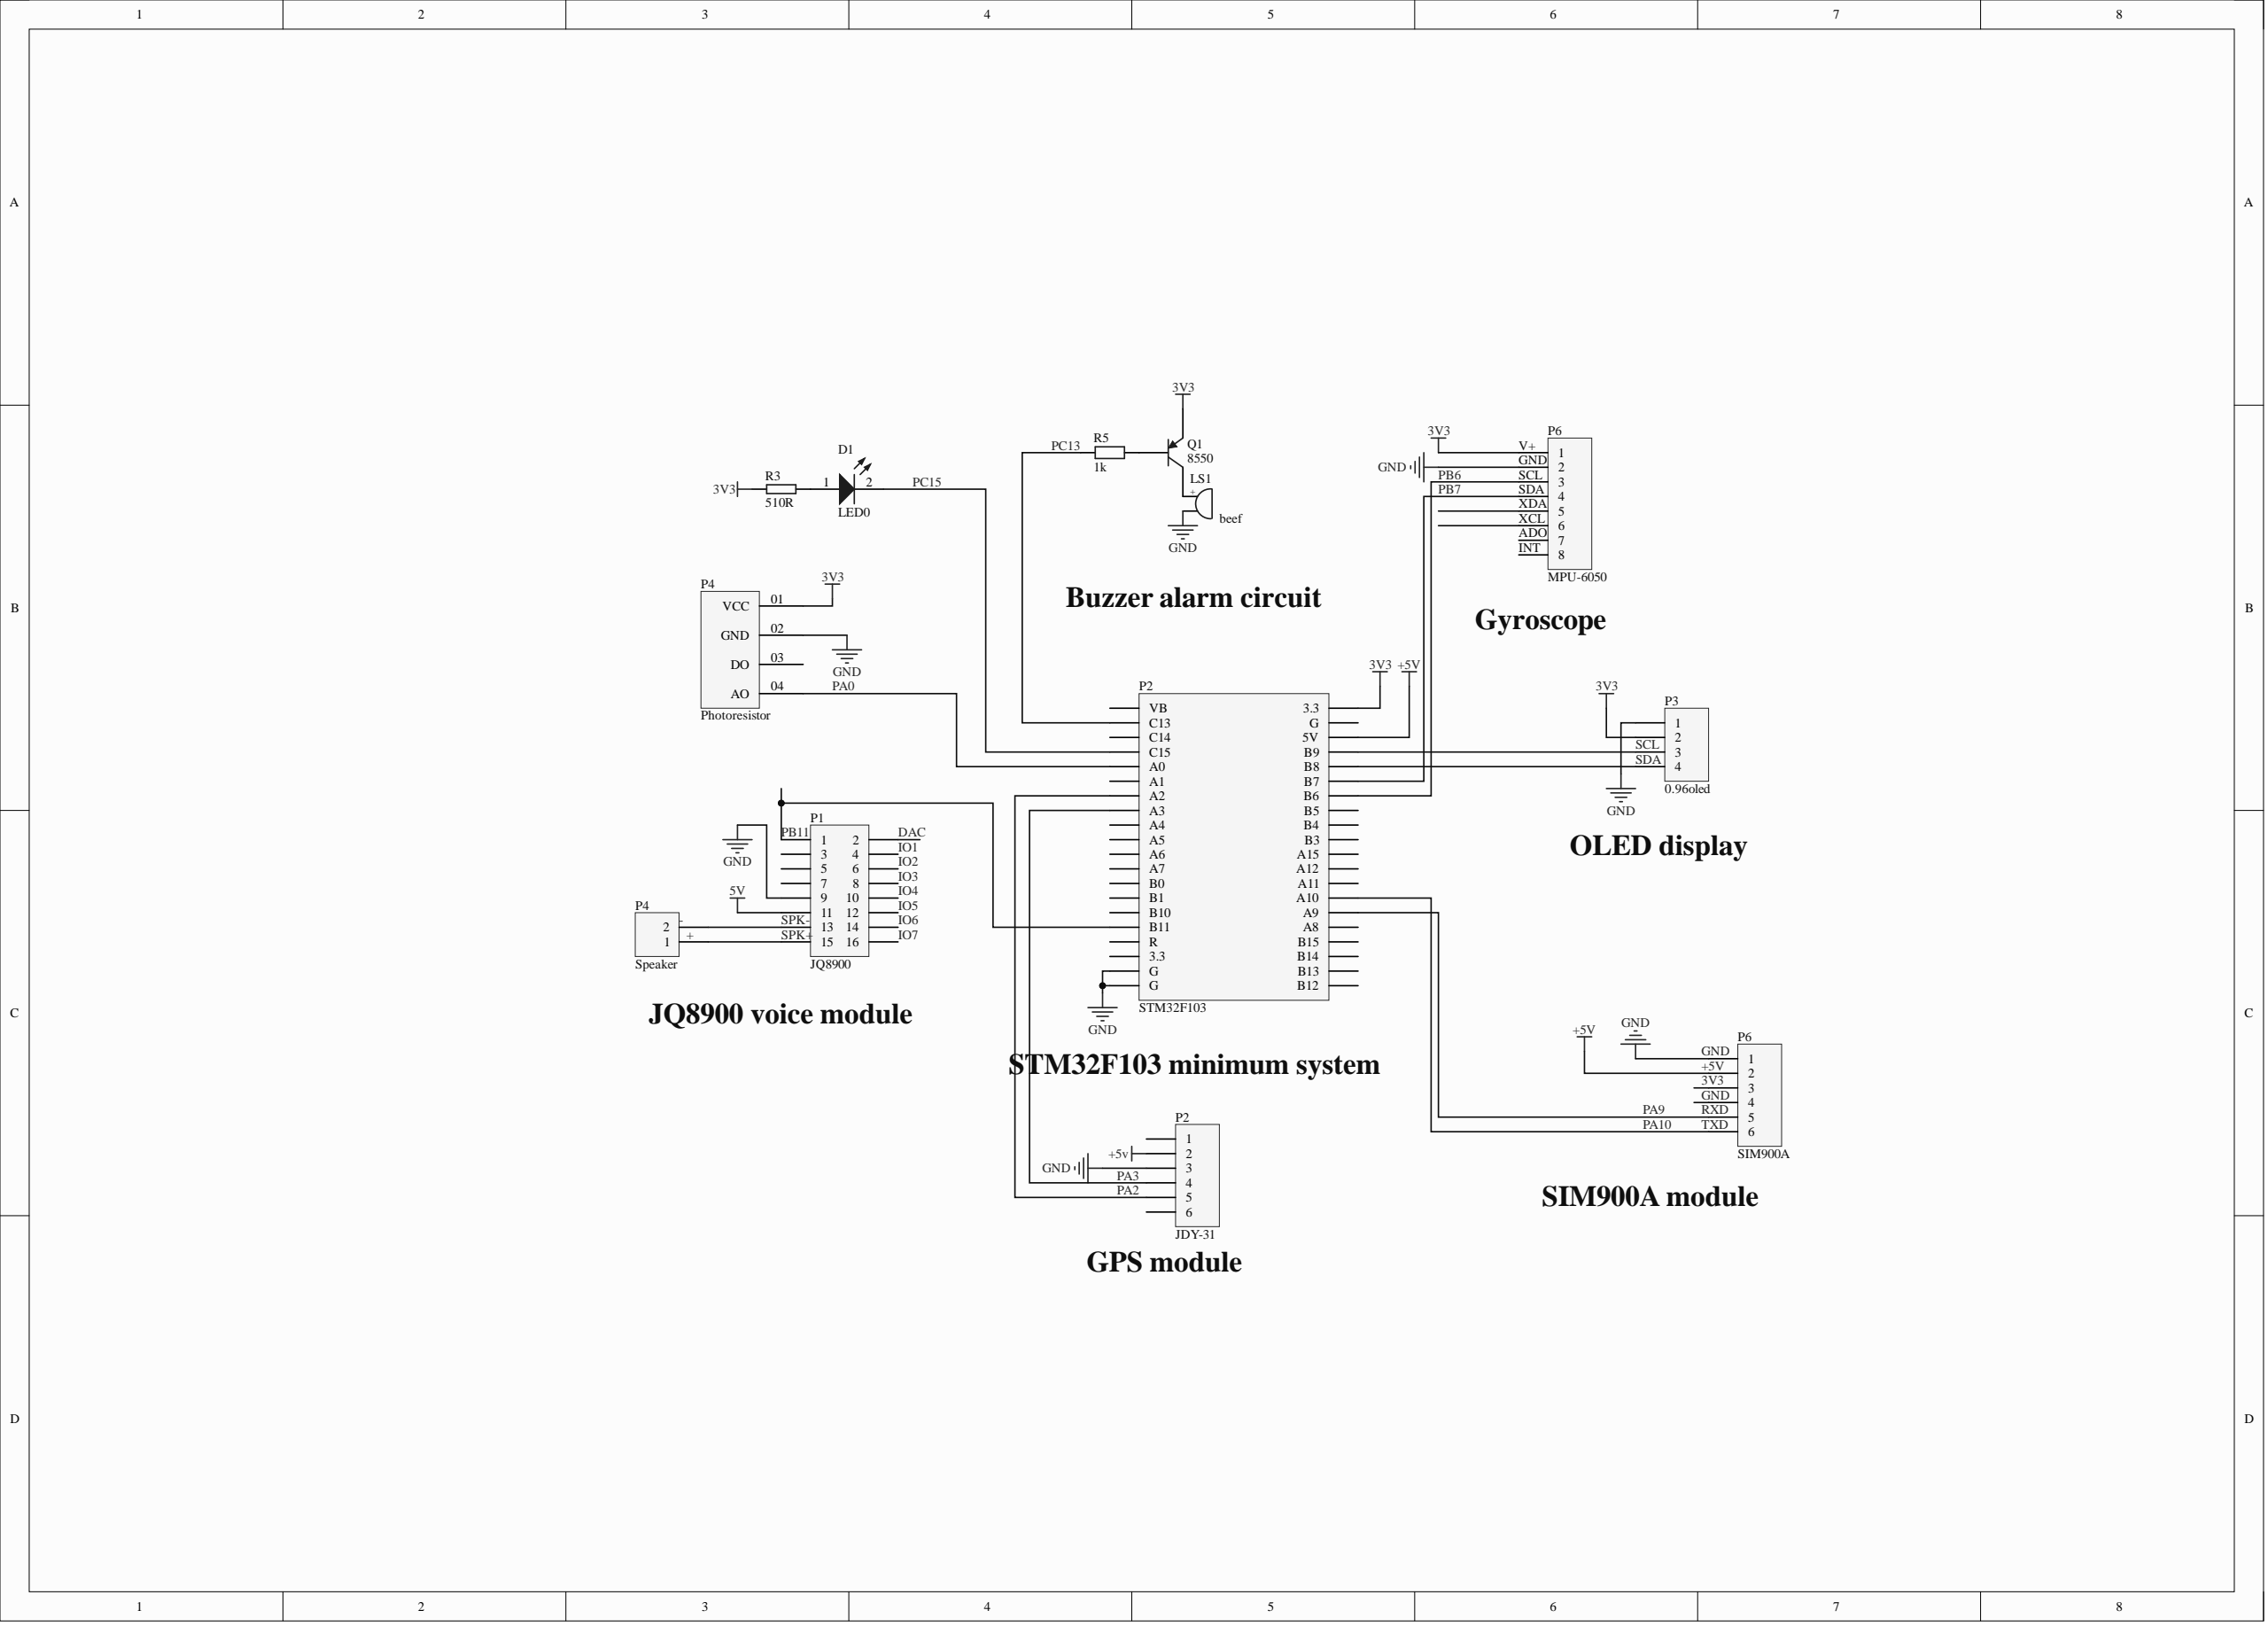Circuit board | Altium Designer | 13 parts | 20 nets
Bill of materials:
Comment,Description,Designator,Footprint,LibRef,Quantity
"LED0","Typical INFRARED GaAs LED","D1","my0603LED","LED0","1"
"beef","Buzzer","LS1","PIN2","BEEP","1"
"JQ8900","Header, 8-Pin, Dual row","P1","HDR2X8","Header 8X2","1"
"JDY-31","Header, 6-Pin","P2","HDR1X6","Header 6","1"
"STM32F103","Header, 20-Pin, Dual row","P2","STM32核心板","Header 20X2","1"
"0.96oled","Header, 4-Pin","P3","HDR1X4","Header 4","1"
"Photoresistor","","P4","HDR1X4","Component_1","1"
"Speaker","Header, 2-Pin","P4","HDR1X2","Header 2","1"
"MPU-6050","Header, 8-Pin","P6","HDR1X8","Header 8","1"
"SIM900A","Header, 6-Pin","P6","HDR1X6","Header 6","1"
"8550","PNP General Purpose Amplifier","Q1","TO-92A","2N3906","1"
"510R","","R3","my0603","R","1"
"1k","SMD resistor","R5","my0603","R","1"
Netlist (Protel format):
[
D1
my0603LED
LED0



]
[
LS1
PIN2
beef



]
[
P1
HDR2X8
JQ8900



]
[
P2
HDR1X6
JDY-31



]
[
P2
STM32核心板
STM32F103



]
[
P3
HDR1X4
0.96oled



]
[
P4
HDR1X4
Photoresistor



]
[
P4
HDR1X2
Speaker



]
[
P6
HDR1X8
MPU-6050



]
[
P6
HDR1X6
SIM900A



]
[
Q1
TO-92A
8550



]
[
R3
my0603
510R



]
[
R5
my0603
1k



]
(
SPK-
P1-13
P4-2
)
(
SPK+
P1-15
P4-1
)
(
SDA
P2-31
P3-4
)
(
SCL
P2-33
P3-3
)
(
PC15
D1-2
P2-34
)
(
PC13
P2-38
R5-1
)
(
PB11
P1-1
P2-10
)
(
PB7
P2-29
P6-4
)
(
PB6
P2-27
P6-3
)
(
PA10
P2-13
P6-6
)
(
PA9
P2-11
P6-5
)
(
PA3
P2-4
P2-26
)
(
PA2
P2-5
P2-28
)
(
PA0
P2-32
P4-04
)
(
NetQ1_2
Q1-2
R5-2
)
(
NetLS1_1
LS1-1
Q1-3
)
(
NetD1_1
D1-1
R3-1
)
(
GND
LS1-2
P1-9
P2-2
P2-3
P2-4
P3-1
P4-02
P6-1
P6-2
P6-4
)
(
+5V
P2-2
P2-35
P6-2
)
(
3V3
P2-39
P3-2
P4-01
P6-1
P6-3
Q1-1
R3-2
)